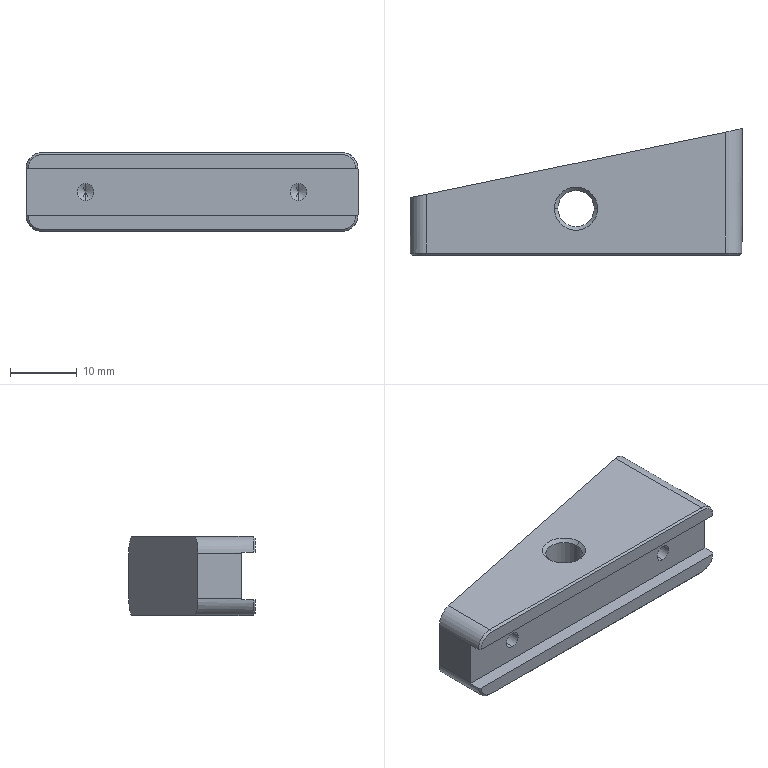Part | STEP file | ND25021-01-JDKM-03-SL | 1 solid | 34 faces | box 49.9 x 19 x 11.9 mm | volume 7050 mm3 | cone 12 | plane 12 | cylinder 10 | commonest cylinder face diameters 2.5 x4 5 x4 5.5 x2